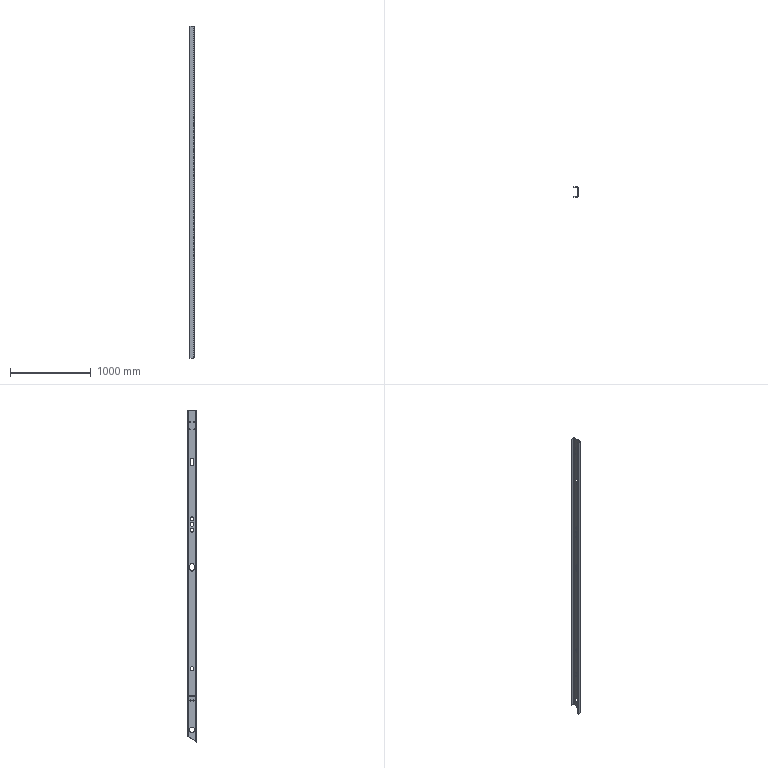Part | SolidWorks | features ICE 4, Cut 2, Extrusion 1 | 1 solid | 50 faces | box 50 x 120 x 4120 mm | volume 4181068 mm3 | cylinder 36 | plane 14 | commonest cylinder face diameters 50 x11 13 x8 16 x8 20 x4 45 x3 65 x2